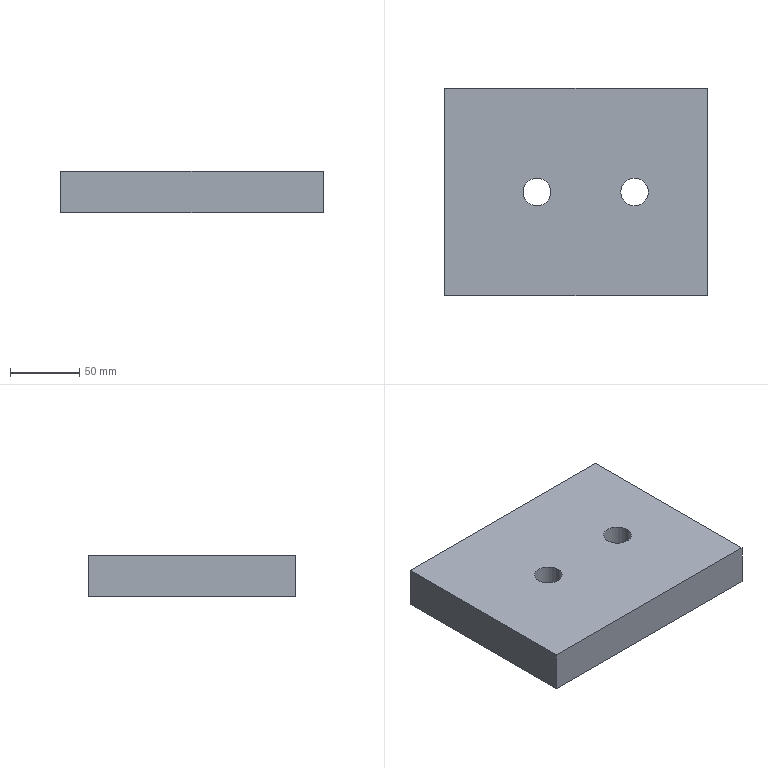Part | STEP file | 1 solid | 10 faces | box 190 x 150 x 30 mm | volume 836150 mm3 | plane 6 | cylinder 4 | commonest cylinder face diameters 20 x4
STEP:
#1=CARTESIAN_POINT('',(0.,0.,0.));
#2=DIRECTION('',(0.,0.,1.));
#3=DIRECTION('',(1.,0.,0.));
#4=AXIS2_PLACEMENT_3D('',#1,#2,#3);
#5=CARTESIAN_POINT('',(-38.283,0.,30.));
#6=VERTEX_POINT('',#5);
#7=CARTESIAN_POINT('',(-38.283,0.,0.));
#8=VERTEX_POINT('',#7);
#9=CARTESIAN_POINT('',(-38.283,0.,-49.));
#10=DIRECTION('',(0.,0.,-1.));
#11=VECTOR('',#10,1.);
#12=LINE('',#9,#11);
#13=CARTESIAN_POINT('',(-28.283,0.,-49.));
#14=DIRECTION('',(0.,0.,-1.));
#15=DIRECTION('',(-1.,0.,0.));
#16=AXIS2_PLACEMENT_3D('',#13,#14,#15);
#17=CYLINDRICAL_SURFACE('',#16,10.);
#18=CARTESIAN_POINT('',(6.283,0.));
#19=DIRECTION('',(0.,1.));
#20=VECTOR('',#19,1.);
#21=LINE('',#18,#20);
#22=(GEOMETRIC_REPRESENTATION_CONTEXT(2)PARAMETRIC_REPRESENTATION_CONTEXT()REPRESENTATION_CONTEXT('',''));
#23=DEFINITIONAL_REPRESENTATION('',(#21),#22);
#24=PCURVE('',#17,#23);
#25=CARTESIAN_POINT('',(-28.283,0.,-49.));
#26=DIRECTION('',(0.,0.,-1.));
#27=DIRECTION('',(-1.,0.,0.));
#28=AXIS2_PLACEMENT_3D('',#25,#26,#27);
#29=CYLINDRICAL_SURFACE('',#28,10.);
#30=CARTESIAN_POINT('',(0.,0.));
#31=DIRECTION('',(0.,1.));
#32=VECTOR('',#31,1.);
#33=LINE('',#30,#32);
#34=(GEOMETRIC_REPRESENTATION_CONTEXT(2)PARAMETRIC_REPRESENTATION_CONTEXT()REPRESENTATION_CONTEXT('',''));
#35=DEFINITIONAL_REPRESENTATION('',(#33),#34);
#36=PCURVE('',#29,#35);
#37=SURFACE_CURVE('',#12,(#24,#36),.PCURVE_S1.);
#38=EDGE_CURVE('',#6,#8,#37,.T.);
#39=ORIENTED_EDGE('',*,*,#38,.T.);
#40=CARTESIAN_POINT('',(-18.283,0.,0.));
#41=VERTEX_POINT('',#40);
#42=CARTESIAN_POINT('',(-28.283,0.,0.));
#43=DIRECTION('',(0.,0.,1.));
#44=DIRECTION('',(-1.,0.,0.));
#45=AXIS2_PLACEMENT_3D('',#42,#43,#44);
#46=CIRCLE('',#45,10.);
#47=CARTESIAN_POINT('',(6.283,-49.));
#48=DIRECTION('',(-1.,0.));
#49=VECTOR('',#48,1.);
#50=LINE('',#47,#49);
#51=(GEOMETRIC_REPRESENTATION_CONTEXT(2)PARAMETRIC_REPRESENTATION_CONTEXT()REPRESENTATION_CONTEXT('',''));
#52=DEFINITIONAL_REPRESENTATION('',(#50),#51);
#53=PCURVE('',#17,#52);
#54=CARTESIAN_POINT('',(0.,0.,0.));
#55=DIRECTION('',(0.,0.,1.));
#56=DIRECTION('',(1.,0.,0.));
#57=AXIS2_PLACEMENT_3D('',#54,#55,#56);
#58=PLANE('',#57);
#59=CARTESIAN_POINT('',(-28.283,0.));
#60=DIRECTION('',(-1.,0.));
#61=AXIS2_PLACEMENT_2D('',#59,#60);
#62=CIRCLE('',#61,10.);
#63=(GEOMETRIC_REPRESENTATION_CONTEXT(2)PARAMETRIC_REPRESENTATION_CONTEXT()REPRESENTATION_CONTEXT('',''));
#64=DEFINITIONAL_REPRESENTATION('',(#62),#63);
#65=PCURVE('',#58,#64);
#66=SURFACE_CURVE('',#46,(#53,#65),.PCURVE_S1.);
#67=EDGE_CURVE('',#8,#41,#66,.T.);
#68=ORIENTED_EDGE('',*,*,#67,.T.);
#69=CARTESIAN_POINT('',(-18.283,0.,30.));
#70=VERTEX_POINT('',#69);
#71=CARTESIAN_POINT('',(-18.283,0.,-49.));
#72=DIRECTION('',(0.,0.,-1.));
#73=VECTOR('',#72,1.);
#74=LINE('',#71,#73);
#75=CARTESIAN_POINT('',(3.142,0.));
#76=DIRECTION('',(0.,1.));
#77=VECTOR('',#76,1.);
#78=LINE('',#75,#77);
#79=(GEOMETRIC_REPRESENTATION_CONTEXT(2)PARAMETRIC_REPRESENTATION_CONTEXT()REPRESENTATION_CONTEXT('',''));
#80=DEFINITIONAL_REPRESENTATION('',(#78),#79);
#81=PCURVE('',#17,#80);
#82=CARTESIAN_POINT('',(3.142,0.));
#83=DIRECTION('',(0.,1.));
#84=VECTOR('',#83,1.);
#85=LINE('',#82,#84);
#86=(GEOMETRIC_REPRESENTATION_CONTEXT(2)PARAMETRIC_REPRESENTATION_CONTEXT()REPRESENTATION_CONTEXT('',''));
#87=DEFINITIONAL_REPRESENTATION('',(#85),#86);
#88=PCURVE('',#29,#87);
#89=SURFACE_CURVE('',#74,(#81,#88),.PCURVE_S1.);
#90=EDGE_CURVE('',#70,#41,#89,.T.);
#91=ORIENTED_EDGE('',*,*,#90,.F.);
#92=CARTESIAN_POINT('',(-28.283,0.,30.));
#93=DIRECTION('',(0.,0.,-1.));
#94=DIRECTION('',(-1.,0.,0.));
#95=AXIS2_PLACEMENT_3D('',#92,#93,#94);
#96=CIRCLE('',#95,10.);
#97=CARTESIAN_POINT('',(0.,-79.));
#98=DIRECTION('',(1.,0.));
#99=VECTOR('',#98,1.);
#100=LINE('',#97,#99);
#101=(GEOMETRIC_REPRESENTATION_CONTEXT(2)PARAMETRIC_REPRESENTATION_CONTEXT()REPRESENTATION_CONTEXT('',''));
#102=DEFINITIONAL_REPRESENTATION('',(#100),#101);
#103=PCURVE('',#17,#102);
#104=CARTESIAN_POINT('',(0.,0.,30.));
#105=DIRECTION('',(0.,0.,1.));
#106=DIRECTION('',(1.,0.,0.));
#107=AXIS2_PLACEMENT_3D('',#104,#105,#106);
#108=PLANE('',#107);
#109=CARTESIAN_POINT('',(-38.283,0.));
#110=CARTESIAN_POINT('',(-38.283,17.321));
#111=CARTESIAN_POINT('',(-23.283,8.66));
#112=CARTESIAN_POINT('',(-8.283,0.));
#113=CARTESIAN_POINT('',(-23.283,-8.66));
#114=CARTESIAN_POINT('',(-38.283,-17.321));
#115=CARTESIAN_POINT('',(-38.283,0.));
#116=(BOUNDED_CURVE()B_SPLINE_CURVE(2,(#109,#110,#111,#112,#113,#114,#115),.UNSPECIFIED.,.T.,.F.)B_SPLINE_CURVE_WITH_KNOTS((1,2,2,2,2,1),(-2.094,0.,2.094,4.189,6.283,8.378),.UNSPECIFIED.)CURVE()GEOMETRIC_REPRESENTATION_ITEM()RATIONAL_B_SPLINE_CURVE((1.,0.5,1.,0.5,1.,0.5,1.))REPRESENTATION_ITEM(''));
#117=(GEOMETRIC_REPRESENTATION_CONTEXT(2)PARAMETRIC_REPRESENTATION_CONTEXT()REPRESENTATION_CONTEXT('',''));
#118=DEFINITIONAL_REPRESENTATION('',(#116),#117);
#119=PCURVE('',#108,#118);
#120=SURFACE_CURVE('',#96,(#103,#119),.PCURVE_S1.);
#121=EDGE_CURVE('',#70,#6,#120,.T.);
#122=ORIENTED_EDGE('',*,*,#121,.T.);
#123=EDGE_LOOP('',(#39,#68,#91,#122));
#124=FACE_BOUND('',#123,.F.);
#125=ADVANCED_FACE('',(#124),#17,.F.);
#126=CARTESIAN_POINT('',(32.428,0.,30.));
#127=VERTEX_POINT('',#126);
#128=CARTESIAN_POINT('',(32.428,0.,0.));
#129=VERTEX_POINT('',#128);
#130=CARTESIAN_POINT('',(32.428,0.,-49.));
#131=DIRECTION('',(0.,0.,-1.));
#132=VECTOR('',#131,1.);
#133=LINE('',#130,#132);
#134=CARTESIAN_POINT('',(42.428,0.,-49.));
#135=DIRECTION('',(0.,0.,-1.));
#136=DIRECTION('',(-1.,0.,0.));
#137=AXIS2_PLACEMENT_3D('',#134,#135,#136);
#138=CYLINDRICAL_SURFACE('',#137,10.);
#139=CARTESIAN_POINT('',(6.283,0.));
#140=DIRECTION('',(0.,1.));
#141=VECTOR('',#140,1.);
#142=LINE('',#139,#141);
#143=(GEOMETRIC_REPRESENTATION_CONTEXT(2)PARAMETRIC_REPRESENTATION_CONTEXT()REPRESENTATION_CONTEXT('',''));
#144=DEFINITIONAL_REPRESENTATION('',(#142),#143);
#145=PCURVE('',#138,#144);
#146=CARTESIAN_POINT('',(42.428,0.,-49.));
#147=DIRECTION('',(0.,0.,-1.));
#148=DIRECTION('',(-1.,0.,0.));
#149=AXIS2_PLACEMENT_3D('',#146,#147,#148);
#150=CYLINDRICAL_SURFACE('',#149,10.);
#151=CARTESIAN_POINT('',(0.,0.));
#152=DIRECTION('',(0.,1.));
#153=VECTOR('',#152,1.);
#154=LINE('',#151,#153);
#155=(GEOMETRIC_REPRESENTATION_CONTEXT(2)PARAMETRIC_REPRESENTATION_CONTEXT()REPRESENTATION_CONTEXT('',''));
#156=DEFINITIONAL_REPRESENTATION('',(#154),#155);
#157=PCURVE('',#150,#156);
#158=SURFACE_CURVE('',#133,(#145,#157),.PCURVE_S1.);
#159=EDGE_CURVE('',#127,#129,#158,.T.);
#160=ORIENTED_EDGE('',*,*,#159,.T.);
#161=CARTESIAN_POINT('',(52.428,0.,0.));
#162=VERTEX_POINT('',#161);
#163=CARTESIAN_POINT('',(42.428,0.,0.));
#164=DIRECTION('',(0.,0.,1.));
#165=DIRECTION('',(-1.,0.,0.));
#166=AXIS2_PLACEMENT_3D('',#163,#164,#165);
#167=CIRCLE('',#166,10.);
#168=CARTESIAN_POINT('',(6.283,-49.));
#169=DIRECTION('',(-1.,0.));
#170=VECTOR('',#169,1.);
#171=LINE('',#168,#170);
#172=(GEOMETRIC_REPRESENTATION_CONTEXT(2)PARAMETRIC_REPRESENTATION_CONTEXT()REPRESENTATION_CONTEXT('',''));
#173=DEFINITIONAL_REPRESENTATION('',(#171),#172);
#174=PCURVE('',#138,#173);
#175=CARTESIAN_POINT('',(42.428,0.));
#176=DIRECTION('',(-1.,0.));
#177=AXIS2_PLACEMENT_2D('',#175,#176);
#178=CIRCLE('',#177,10.);
#179=(GEOMETRIC_REPRESENTATION_CONTEXT(2)PARAMETRIC_REPRESENTATION_CONTEXT()REPRESENTATION_CONTEXT('',''));
#180=DEFINITIONAL_REPRESENTATION('',(#178),#179);
#181=PCURVE('',#58,#180);
#182=SURFACE_CURVE('',#167,(#174,#181),.PCURVE_S1.);
#183=EDGE_CURVE('',#129,#162,#182,.T.);
#184=ORIENTED_EDGE('',*,*,#183,.T.);
#185=CARTESIAN_POINT('',(52.428,0.,30.));
#186=VERTEX_POINT('',#185);
#187=CARTESIAN_POINT('',(52.428,0.,-49.));
#188=DIRECTION('',(0.,0.,-1.));
#189=VECTOR('',#188,1.);
#190=LINE('',#187,#189);
#191=CARTESIAN_POINT('',(3.142,0.));
#192=DIRECTION('',(0.,1.));
#193=VECTOR('',#192,1.);
#194=LINE('',#191,#193);
#195=(GEOMETRIC_REPRESENTATION_CONTEXT(2)PARAMETRIC_REPRESENTATION_CONTEXT()REPRESENTATION_CONTEXT('',''));
#196=DEFINITIONAL_REPRESENTATION('',(#194),#195);
#197=PCURVE('',#138,#196);
#198=CARTESIAN_POINT('',(3.142,0.));
#199=DIRECTION('',(0.,1.));
#200=VECTOR('',#199,1.);
#201=LINE('',#198,#200);
#202=(GEOMETRIC_REPRESENTATION_CONTEXT(2)PARAMETRIC_REPRESENTATION_CONTEXT()REPRESENTATION_CONTEXT('',''));
#203=DEFINITIONAL_REPRESENTATION('',(#201),#202);
#204=PCURVE('',#150,#203);
#205=SURFACE_CURVE('',#190,(#197,#204),.PCURVE_S1.);
#206=EDGE_CURVE('',#186,#162,#205,.T.);
#207=ORIENTED_EDGE('',*,*,#206,.F.);
#208=CARTESIAN_POINT('',(42.428,0.,30.));
#209=DIRECTION('',(0.,0.,-1.));
#210=DIRECTION('',(-1.,0.,0.));
#211=AXIS2_PLACEMENT_3D('',#208,#209,#210);
#212=CIRCLE('',#211,10.);
#213=CARTESIAN_POINT('',(0.,-79.));
#214=DIRECTION('',(1.,0.));
#215=VECTOR('',#214,1.);
#216=LINE('',#213,#215);
#217=(GEOMETRIC_REPRESENTATION_CONTEXT(2)PARAMETRIC_REPRESENTATION_CONTEXT()REPRESENTATION_CONTEXT('',''));
#218=DEFINITIONAL_REPRESENTATION('',(#216),#217);
#219=PCURVE('',#138,#218);
#220=CARTESIAN_POINT('',(32.428,0.));
#221=CARTESIAN_POINT('',(32.428,17.321));
#222=CARTESIAN_POINT('',(47.428,8.66));
#223=CARTESIAN_POINT('',(62.428,0.));
#224=CARTESIAN_POINT('',(47.428,-8.66));
#225=CARTESIAN_POINT('',(32.428,-17.321));
#226=CARTESIAN_POINT('',(32.428,0.));
#227=(BOUNDED_CURVE()B_SPLINE_CURVE(2,(#220,#221,#222,#223,#224,#225,#226),.UNSPECIFIED.,.T.,.F.)B_SPLINE_CURVE_WITH_KNOTS((1,2,2,2,2,1),(-2.094,0.,2.094,4.189,6.283,8.378),.UNSPECIFIED.)CURVE()GEOMETRIC_REPRESENTATION_ITEM()RATIONAL_B_SPLINE_CURVE((1.,0.5,1.,0.5,1.,0.5,1.))REPRESENTATION_ITEM(''));
#228=(GEOMETRIC_REPRESENTATION_CONTEXT(2)PARAMETRIC_REPRESENTATION_CONTEXT()REPRESENTATION_CONTEXT('',''));
#229=DEFINITIONAL_REPRESENTATION('',(#227),#228);
#230=PCURVE('',#108,#229);
#231=SURFACE_CURVE('',#212,(#219,#230),.PCURVE_S1.);
#232=EDGE_CURVE('',#186,#127,#231,.T.);
#233=ORIENTED_EDGE('',*,*,#232,.T.);
#234=EDGE_LOOP('',(#160,#184,#207,#233));
#235=FACE_BOUND('',#234,.F.);
#236=ADVANCED_FACE('',(#235),#138,.F.);
#237=CARTESIAN_POINT('',(-28.283,0.,30.));
#238=DIRECTION('',(0.,0.,-1.));
#239=DIRECTION('',(-1.,0.,0.));
#240=AXIS2_PLACEMENT_3D('',#237,#238,#239);
#241=CIRCLE('',#240,10.);
#242=CARTESIAN_POINT('',(-38.283,0.));
#243=CARTESIAN_POINT('',(-38.283,17.321));
#244=CARTESIAN_POINT('',(-23.283,8.66));
#245=CARTESIAN_POINT('',(-8.283,0.));
#246=CARTESIAN_POINT('',(-23.283,-8.66));
#247=CARTESIAN_POINT('',(-38.283,-17.321));
#248=CARTESIAN_POINT('',(-38.283,0.));
#249=(BOUNDED_CURVE()B_SPLINE_CURVE(2,(#242,#243,#244,#245,#246,#247,#248),.UNSPECIFIED.,.T.,.F.)B_SPLINE_CURVE_WITH_KNOTS((1,2,2,2,2,1),(-2.094,0.,2.094,4.189,6.283,8.378),.UNSPECIFIED.)CURVE()GEOMETRIC_REPRESENTATION_ITEM()RATIONAL_B_SPLINE_CURVE((1.,0.5,1.,0.5,1.,0.5,1.))REPRESENTATION_ITEM(''));
#250=(GEOMETRIC_REPRESENTATION_CONTEXT(2)PARAMETRIC_REPRESENTATION_CONTEXT()REPRESENTATION_CONTEXT('',''));
#251=DEFINITIONAL_REPRESENTATION('',(#249),#250);
#252=PCURVE('',#108,#251);
#253=CARTESIAN_POINT('',(0.,-79.));
#254=DIRECTION('',(1.,0.));
#255=VECTOR('',#254,1.);
#256=LINE('',#253,#255);
#257=(GEOMETRIC_REPRESENTATION_CONTEXT(2)PARAMETRIC_REPRESENTATION_CONTEXT()REPRESENTATION_CONTEXT('',''));
#258=DEFINITIONAL_REPRESENTATION('',(#256),#257);
#259=PCURVE('',#29,#258);
#260=SURFACE_CURVE('',#241,(#252,#259),.PCURVE_S1.);
#261=EDGE_CURVE('',#6,#70,#260,.T.);
#262=ORIENTED_EDGE('',*,*,#261,.T.);
#263=ORIENTED_EDGE('',*,*,#121,.T.);
#264=EDGE_LOOP('',(#262,#263));
#265=FACE_BOUND('',#264,.T.);
#266=CARTESIAN_POINT('',(42.428,0.,30.));
#267=DIRECTION('',(0.,0.,-1.));
#268=DIRECTION('',(-1.,0.,0.));
#269=AXIS2_PLACEMENT_3D('',#266,#267,#268);
#270=CIRCLE('',#269,10.);
#271=CARTESIAN_POINT('',(32.428,0.));
#272=CARTESIAN_POINT('',(32.428,17.321));
#273=CARTESIAN_POINT('',(47.428,8.66));
#274=CARTESIAN_POINT('',(62.428,0.));
#275=CARTESIAN_POINT('',(47.428,-8.66));
#276=CARTESIAN_POINT('',(32.428,-17.321));
#277=CARTESIAN_POINT('',(32.428,0.));
#278=(BOUNDED_CURVE()B_SPLINE_CURVE(2,(#271,#272,#273,#274,#275,#276,#277),.UNSPECIFIED.,.T.,.F.)B_SPLINE_CURVE_WITH_KNOTS((1,2,2,2,2,1),(-2.094,0.,2.094,4.189,6.283,8.378),.UNSPECIFIED.)CURVE()GEOMETRIC_REPRESENTATION_ITEM()RATIONAL_B_SPLINE_CURVE((1.,0.5,1.,0.5,1.,0.5,1.))REPRESENTATION_ITEM(''));
#279=(GEOMETRIC_REPRESENTATION_CONTEXT(2)PARAMETRIC_REPRESENTATION_CONTEXT()REPRESENTATION_CONTEXT('',''));
#280=DEFINITIONAL_REPRESENTATION('',(#278),#279);
#281=PCURVE('',#108,#280);
#282=CARTESIAN_POINT('',(0.,-79.));
#283=DIRECTION('',(1.,0.));
#284=VECTOR('',#283,1.);
#285=LINE('',#282,#284);
#286=(GEOMETRIC_REPRESENTATION_CONTEXT(2)PARAMETRIC_REPRESENTATION_CONTEXT()REPRESENTATION_CONTEXT('',''));
#287=DEFINITIONAL_REPRESENTATION('',(#285),#286);
#288=PCURVE('',#150,#287);
#289=SURFACE_CURVE('',#270,(#281,#288),.PCURVE_S1.);
#290=EDGE_CURVE('',#127,#186,#289,.T.);
#291=ORIENTED_EDGE('',*,*,#290,.T.);
#292=ORIENTED_EDGE('',*,*,#232,.T.);
#293=EDGE_LOOP('',(#291,#292));
#294=FACE_BOUND('',#293,.T.);
#295=CARTESIAN_POINT('',(-95.,75.,30.));
#296=VERTEX_POINT('',#295);
#297=CARTESIAN_POINT('',(-95.,-75.,30.));
#298=VERTEX_POINT('',#297);
#299=CARTESIAN_POINT('',(-95.,0.,30.));
#300=DIRECTION('',(0.,-1.,0.));
#301=VECTOR('',#300,1.);
#302=LINE('',#299,#301);
#303=CARTESIAN_POINT('',(-95.,0.));
#304=DIRECTION('',(0.,-1.));
#305=VECTOR('',#304,1.);
#306=LINE('',#303,#305);
#307=(GEOMETRIC_REPRESENTATION_CONTEXT(2)PARAMETRIC_REPRESENTATION_CONTEXT()REPRESENTATION_CONTEXT('',''));
#308=DEFINITIONAL_REPRESENTATION('',(#306),#307);
#309=PCURVE('',#108,#308);
#310=CARTESIAN_POINT('',(-95.,75.,30.));
#311=DIRECTION('',(1.,0.,0.));
#312=DIRECTION('',(0.,1.,0.));
#313=AXIS2_PLACEMENT_3D('',#310,#311,#312);
#314=PLANE('',#313);
#315=CARTESIAN_POINT('',(-75.,0.));
#316=DIRECTION('',(-1.,0.));
#317=VECTOR('',#316,1.);
#318=LINE('',#315,#317);
#319=(GEOMETRIC_REPRESENTATION_CONTEXT(2)PARAMETRIC_REPRESENTATION_CONTEXT()REPRESENTATION_CONTEXT('',''));
#320=DEFINITIONAL_REPRESENTATION('',(#318),#319);
#321=PCURVE('',#314,#320);
#322=SURFACE_CURVE('',#302,(#309,#321),.PCURVE_S1.);
#323=EDGE_CURVE('',#296,#298,#322,.T.);
#324=ORIENTED_EDGE('',*,*,#323,.T.);
#325=CARTESIAN_POINT('',(95.,-75.,30.));
#326=VERTEX_POINT('',#325);
#327=CARTESIAN_POINT('',(0.,-75.,30.));
#328=DIRECTION('',(1.,0.,0.));
#329=VECTOR('',#328,1.);
#330=LINE('',#327,#329);
#331=CARTESIAN_POINT('',(0.,-75.));
#332=DIRECTION('',(1.,0.));
#333=VECTOR('',#332,1.);
#334=LINE('',#331,#333);
#335=(GEOMETRIC_REPRESENTATION_CONTEXT(2)PARAMETRIC_REPRESENTATION_CONTEXT()REPRESENTATION_CONTEXT('',''));
#336=DEFINITIONAL_REPRESENTATION('',(#334),#335);
#337=PCURVE('',#108,#336);
#338=CARTESIAN_POINT('',(-95.,-75.,30.));
#339=DIRECTION('',(0.,1.,0.));
#340=DIRECTION('',(0.,0.,1.));
#341=AXIS2_PLACEMENT_3D('',#338,#339,#340);
#342=PLANE('',#341);
#343=CARTESIAN_POINT('',(0.,95.));
#344=DIRECTION('',(0.,1.));
#345=VECTOR('',#344,1.);
#346=LINE('',#343,#345);
#347=(GEOMETRIC_REPRESENTATION_CONTEXT(2)PARAMETRIC_REPRESENTATION_CONTEXT()REPRESENTATION_CONTEXT('',''));
#348=DEFINITIONAL_REPRESENTATION('',(#346),#347);
#349=PCURVE('',#342,#348);
#350=SURFACE_CURVE('',#330,(#337,#349),.PCURVE_S1.);
#351=EDGE_CURVE('',#298,#326,#350,.T.);
#352=ORIENTED_EDGE('',*,*,#351,.T.);
#353=CARTESIAN_POINT('',(95.,75.,30.));
#354=VERTEX_POINT('',#353);
#355=CARTESIAN_POINT('',(95.,0.,30.));
#356=DIRECTION('',(0.,1.,0.));
#357=VECTOR('',#356,1.);
#358=LINE('',#355,#357);
#359=CARTESIAN_POINT('',(95.,0.));
#360=DIRECTION('',(0.,1.));
#361=VECTOR('',#360,1.);
#362=LINE('',#359,#361);
#363=(GEOMETRIC_REPRESENTATION_CONTEXT(2)PARAMETRIC_REPRESENTATION_CONTEXT()REPRESENTATION_CONTEXT('',''));
#364=DEFINITIONAL_REPRESENTATION('',(#362),#363);
#365=PCURVE('',#108,#364);
#366=CARTESIAN_POINT('',(95.,75.,30.));
#367=DIRECTION('',(-1.,0.,0.));
#368=DIRECTION('',(0.,0.,1.));
#369=AXIS2_PLACEMENT_3D('',#366,#367,#368);
#370=PLANE('',#369);
#371=CARTESIAN_POINT('',(0.,-75.));
#372=DIRECTION('',(0.,1.));
#373=VECTOR('',#372,1.);
#374=LINE('',#371,#373);
#375=(GEOMETRIC_REPRESENTATION_CONTEXT(2)PARAMETRIC_REPRESENTATION_CONTEXT()REPRESENTATION_CONTEXT('',''));
#376=DEFINITIONAL_REPRESENTATION('',(#374),#375);
#377=PCURVE('',#370,#376);
#378=SURFACE_CURVE('',#358,(#365,#377),.PCURVE_S1.);
#379=EDGE_CURVE('',#326,#354,#378,.T.);
#380=ORIENTED_EDGE('',*,*,#379,.T.);
#381=CARTESIAN_POINT('',(0.,75.,30.));
#382=DIRECTION('',(-1.,0.,0.));
#383=VECTOR('',#382,1.);
#384=LINE('',#381,#383);
#385=CARTESIAN_POINT('',(0.,75.));
#386=DIRECTION('',(-1.,0.));
#387=VECTOR('',#386,1.);
#388=LINE('',#385,#387);
#389=(GEOMETRIC_REPRESENTATION_CONTEXT(2)PARAMETRIC_REPRESENTATION_CONTEXT()REPRESENTATION_CONTEXT('',''));
#390=DEFINITIONAL_REPRESENTATION('',(#388),#389);
#391=PCURVE('',#108,#390);
#392=CARTESIAN_POINT('',(-95.,75.,30.));
#393=DIRECTION('',(0.,-1.,0.));
#394=DIRECTION('',(0.,0.,-1.));
#395=AXIS2_PLACEMENT_3D('',#392,#393,#394);
#396=PLANE('',#395);
#397=CARTESIAN_POINT('',(0.,95.));
#398=DIRECTION('',(0.,-1.));
#399=VECTOR('',#398,1.);
#400=LINE('',#397,#399);
#401=(GEOMETRIC_REPRESENTATION_CONTEXT(2)PARAMETRIC_REPRESENTATION_CONTEXT()REPRESENTATION_CONTEXT('',''));
#402=DEFINITIONAL_REPRESENTATION('',(#400),#401);
#403=PCURVE('',#396,#402);
#404=SURFACE_CURVE('',#384,(#391,#403),.PCURVE_S1.);
#405=EDGE_CURVE('',#354,#296,#404,.T.);
#406=ORIENTED_EDGE('',*,*,#405,.T.);
#407=EDGE_LOOP('',(#324,#352,#380,#406));
#408=FACE_BOUND('',#407,.T.);
#409=ADVANCED_FACE('',(#265,#294,#408),#108,.T.);
#410=CARTESIAN_POINT('',(-28.283,0.,0.));
#411=DIRECTION('',(0.,0.,1.));
#412=DIRECTION('',(-1.,0.,0.));
#413=AXIS2_PLACEMENT_3D('',#410,#411,#412);
#414=CIRCLE('',#413,10.);
#415=CARTESIAN_POINT('',(6.283,-49.));
#416=DIRECTION('',(-1.,0.));
#417=VECTOR('',#416,1.);
#418=LINE('',#415,#417);
#419=(GEOMETRIC_REPRESENTATION_CONTEXT(2)PARAMETRIC_REPRESENTATION_CONTEXT()REPRESENTATION_CONTEXT('',''));
#420=DEFINITIONAL_REPRESENTATION('',(#418),#419);
#421=PCURVE('',#29,#420);
#422=CARTESIAN_POINT('',(-28.283,0.));
#423=DIRECTION('',(-1.,0.));
#424=AXIS2_PLACEMENT_2D('',#422,#423);
#425=CIRCLE('',#424,10.);
#426=(GEOMETRIC_REPRESENTATION_CONTEXT(2)PARAMETRIC_REPRESENTATION_CONTEXT()REPRESENTATION_CONTEXT('',''));
#427=DEFINITIONAL_REPRESENTATION('',(#425),#426);
#428=PCURVE('',#58,#427);
#429=SURFACE_CURVE('',#414,(#421,#428),.PCURVE_S1.);
#430=EDGE_CURVE('',#41,#8,#429,.T.);
#431=ORIENTED_EDGE('',*,*,#430,.T.);
#432=ORIENTED_EDGE('',*,*,#38,.F.);
#433=ORIENTED_EDGE('',*,*,#261,.T.);
#434=ORIENTED_EDGE('',*,*,#90,.T.);
#435=EDGE_LOOP('',(#431,#432,#433,#434));
#436=FACE_BOUND('',#435,.F.);
#437=ADVANCED_FACE('',(#436),#29,.F.);
#438=CARTESIAN_POINT('',(42.428,0.,0.));
#439=DIRECTION('',(0.,0.,1.));
#440=DIRECTION('',(-1.,0.,0.));
#441=AXIS2_PLACEMENT_3D('',#438,#439,#440);
#442=CIRCLE('',#441,10.);
#443=CARTESIAN_POINT('',(6.283,-49.));
#444=DIRECTION('',(-1.,0.));
#445=VECTOR('',#444,1.);
#446=LINE('',#443,#445);
#447=(GEOMETRIC_REPRESENTATION_CONTEXT(2)PARAMETRIC_REPRESENTATION_CONTEXT()REPRESENTATION_CONTEXT('',''));
#448=DEFINITIONAL_REPRESENTATION('',(#446),#447);
#449=PCURVE('',#150,#448);
#450=CARTESIAN_POINT('',(42.428,0.));
#451=DIRECTION('',(-1.,0.));
#452=AXIS2_PLACEMENT_2D('',#450,#451);
#453=CIRCLE('',#452,10.);
#454=(GEOMETRIC_REPRESENTATION_CONTEXT(2)PARAMETRIC_REPRESENTATION_CONTEXT()REPRESENTATION_CONTEXT('',''));
#455=DEFINITIONAL_REPRESENTATION('',(#453),#454);
#456=PCURVE('',#58,#455);
#457=SURFACE_CURVE('',#442,(#449,#456),.PCURVE_S1.);
#458=EDGE_CURVE('',#162,#129,#457,.T.);
#459=ORIENTED_EDGE('',*,*,#458,.T.);
#460=ORIENTED_EDGE('',*,*,#159,.F.);
#461=ORIENTED_EDGE('',*,*,#290,.T.);
#462=ORIENTED_EDGE('',*,*,#206,.T.);
#463=EDGE_LOOP('',(#459,#460,#461,#462));
#464=FACE_BOUND('',#463,.F.);
#465=ADVANCED_FACE('',(#464),#150,.F.);
#466=CARTESIAN_POINT('',(95.,-75.,0.));
#467=VERTEX_POINT('',#466);
#468=CARTESIAN_POINT('',(95.,-75.,30.));
#469=DIRECTION('',(0.,0.,-1.));
#470=VECTOR('',#469,1.);
#471=LINE('',#468,#470);
#472=CARTESIAN_POINT('',(0.,190.));
#473=DIRECTION('',(-1.,0.));
#474=VECTOR('',#473,1.);
#475=LINE('',#472,#474);
#476=(GEOMETRIC_REPRESENTATION_CONTEXT(2)PARAMETRIC_REPRESENTATION_CONTEXT()REPRESENTATION_CONTEXT('',''));
#477=DEFINITIONAL_REPRESENTATION('',(#475),#476);
#478=PCURVE('',#342,#477);
#479=CARTESIAN_POINT('',(0.,-150.));
#480=DIRECTION('',(-1.,0.));
#481=VECTOR('',#480,1.);
#482=LINE('',#479,#481);
#483=(GEOMETRIC_REPRESENTATION_CONTEXT(2)PARAMETRIC_REPRESENTATION_CONTEXT()REPRESENTATION_CONTEXT('',''));
#484=DEFINITIONAL_REPRESENTATION('',(#482),#483);
#485=PCURVE('',#370,#484);
#486=SURFACE_CURVE('',#471,(#478,#485),.PCURVE_S1.);
#487=EDGE_CURVE('',#326,#467,#486,.T.);
#488=ORIENTED_EDGE('',*,*,#487,.F.);
#489=ORIENTED_EDGE('',*,*,#351,.F.);
#490=CARTESIAN_POINT('',(-95.,-75.,0.));
#491=VERTEX_POINT('',#490);
#492=CARTESIAN_POINT('',(-95.,-75.,30.));
#493=DIRECTION('',(0.,0.,1.));
#494=VECTOR('',#493,1.);
#495=LINE('',#492,#494);
#496=CARTESIAN_POINT('',(0.,0.));
#497=DIRECTION('',(1.,0.));
#498=VECTOR('',#497,1.);
#499=LINE('',#496,#498);
#500=(GEOMETRIC_REPRESENTATION_CONTEXT(2)PARAMETRIC_REPRESENTATION_CONTEXT()REPRESENTATION_CONTEXT('',''));
#501=DEFINITIONAL_REPRESENTATION('',(#499),#500);
#502=PCURVE('',#342,#501);
#503=CARTESIAN_POINT('',(-150.,0.));
#504=DIRECTION('',(0.,1.));
#505=VECTOR('',#504,1.);
#506=LINE('',#503,#505);
#507=(GEOMETRIC_REPRESENTATION_CONTEXT(2)PARAMETRIC_REPRESENTATION_CONTEXT()REPRESENTATION_CONTEXT('',''));
#508=DEFINITIONAL_REPRESENTATION('',(#506),#507);
#509=PCURVE('',#314,#508);
#510=SURFACE_CURVE('',#495,(#502,#509),.PCURVE_S1.);
#511=EDGE_CURVE('',#491,#298,#510,.T.);
#512=ORIENTED_EDGE('',*,*,#511,.F.);
#513=CARTESIAN_POINT('',(-95.,-75.,0.));
#514=DIRECTION('',(-1.,0.,0.));
#515=VECTOR('',#514,1.);
#516=LINE('',#513,#515);
#517=CARTESIAN_POINT('',(-30.,0.));
#518=DIRECTION('',(0.,-1.));
#519=VECTOR('',#518,1.);
#520=LINE('',#517,#519);
#521=(GEOMETRIC_REPRESENTATION_CONTEXT(2)PARAMETRIC_REPRESENTATION_CONTEXT()REPRESENTATION_CONTEXT('',''));
#522=DEFINITIONAL_REPRESENTATION('',(#520),#521);
#523=PCURVE('',#342,#522);
#524=CARTESIAN_POINT('',(-95.,-75.));
#525=DIRECTION('',(-1.,0.));
#526=VECTOR('',#525,1.);
#527=LINE('',#524,#526);
#528=(GEOMETRIC_REPRESENTATION_CONTEXT(2)PARAMETRIC_REPRESENTATION_CONTEXT()REPRESENTATION_CONTEXT('',''));
#529=DEFINITIONAL_REPRESENTATION('',(#527),#528);
#530=PCURVE('',#58,#529);
#531=SURFACE_CURVE('',#516,(#523,#530),.PCURVE_S1.);
#532=EDGE_CURVE('',#467,#491,#531,.T.);
#533=ORIENTED_EDGE('',*,*,#532,.F.);
#534=EDGE_LOOP('',(#488,#489,#512,#533));
#535=FACE_BOUND('',#534,.T.);
#536=ADVANCED_FACE('',(#535),#342,.F.);
#537=ORIENTED_EDGE('',*,*,#511,.T.);
#538=ORIENTED_EDGE('',*,*,#323,.F.);
#539=CARTESIAN_POINT('',(-95.,75.,0.));
#540=VERTEX_POINT('',#539);
#541=CARTESIAN_POINT('',(-95.,75.,30.));
#542=DIRECTION('',(0.,0.,1.));
#543=VECTOR('',#542,1.);
#544=LINE('',#541,#543);
#545=CARTESIAN_POINT('',(0.,0.));
#546=DIRECTION('',(0.,1.));
#547=VECTOR('',#546,1.);
#548=LINE('',#545,#547);
#549=(GEOMETRIC_REPRESENTATION_CONTEXT(2)PARAMETRIC_REPRESENTATION_CONTEXT()REPRESENTATION_CONTEXT('',''));
#550=DEFINITIONAL_REPRESENTATION('',(#548),#549);
#551=PCURVE('',#314,#550);
#552=CARTESIAN_POINT('',(0.,0.));
#553=DIRECTION('',(-1.,0.));
#554=VECTOR('',#553,1.);
#555=LINE('',#552,#554);
#556=(GEOMETRIC_REPRESENTATION_CONTEXT(2)PARAMETRIC_REPRESENTATION_CONTEXT()REPRESENTATION_CONTEXT('',''));
#557=DEFINITIONAL_REPRESENTATION('',(#555),#556);
#558=PCURVE('',#396,#557);
#559=SURFACE_CURVE('',#544,(#551,#558),.PCURVE_S1.);
#560=EDGE_CURVE('',#540,#296,#559,.T.);
#561=ORIENTED_EDGE('',*,*,#560,.F.);
#562=CARTESIAN_POINT('',(-95.,75.,0.));
#563=DIRECTION('',(0.,1.,0.));
#564=VECTOR('',#563,1.);
#565=LINE('',#562,#564);
#566=CARTESIAN_POINT('',(0.,-30.));
#567=DIRECTION('',(1.,0.));
#568=VECTOR('',#567,1.);
#569=LINE('',#566,#568);
#570=(GEOMETRIC_REPRESENTATION_CONTEXT(2)PARAMETRIC_REPRESENTATION_CONTEXT()REPRESENTATION_CONTEXT('',''));
#571=DEFINITIONAL_REPRESENTATION('',(#569),#570);
#572=PCURVE('',#314,#571);
#573=CARTESIAN_POINT('',(-95.,75.));
#574=DIRECTION('',(0.,1.));
#575=VECTOR('',#574,1.);
#576=LINE('',#573,#575);
#577=(GEOMETRIC_REPRESENTATION_CONTEXT(2)PARAMETRIC_REPRESENTATION_CONTEXT()REPRESENTATION_CONTEXT('',''));
#578=DEFINITIONAL_REPRESENTATION('',(#576),#577);
#579=PCURVE('',#58,#578);
#580=SURFACE_CURVE('',#565,(#572,#579),.PCURVE_S1.);
#581=EDGE_CURVE('',#491,#540,#580,.T.);
#582=ORIENTED_EDGE('',*,*,#581,.F.);
#583=EDGE_LOOP('',(#537,#538,#561,#582));
#584=FACE_BOUND('',#583,.T.);
#585=ADVANCED_FACE('',(#584),#314,.F.);
#586=ORIENTED_EDGE('',*,*,#560,.T.);
#587=ORIENTED_EDGE('',*,*,#405,.F.);
#588=CARTESIAN_POINT('',(95.,75.,0.));
#589=VERTEX_POINT('',#588);
#590=CARTESIAN_POINT('',(95.,75.,30.));
#591=DIRECTION('',(0.,0.,1.));
#592=VECTOR('',#591,1.);
#593=LINE('',#590,#592);
#594=CARTESIAN_POINT('',(0.,190.));
#595=DIRECTION('',(-1.,0.));
#596=VECTOR('',#595,1.);
#597=LINE('',#594,#596);
#598=(GEOMETRIC_REPRESENTATION_CONTEXT(2)PARAMETRIC_REPRESENTATION_CONTEXT()REPRESENTATION_CONTEXT('',''));
#599=DEFINITIONAL_REPRESENTATION('',(#597),#598);
#600=PCURVE('',#396,#599);
#601=CARTESIAN_POINT('',(0.,0.));
#602=DIRECTION('',(1.,0.));
#603=VECTOR('',#602,1.);
#604=LINE('',#601,#603);
#605=(GEOMETRIC_REPRESENTATION_CONTEXT(2)PARAMETRIC_REPRESENTATION_CONTEXT()REPRESENTATION_CONTEXT('',''));
#606=DEFINITIONAL_REPRESENTATION('',(#604),#605);
#607=PCURVE('',#370,#606);
#608=SURFACE_CURVE('',#593,(#600,#607),.PCURVE_S1.);
#609=EDGE_CURVE('',#589,#354,#608,.T.);
#610=ORIENTED_EDGE('',*,*,#609,.F.);
#611=CARTESIAN_POINT('',(-95.,75.,0.));
#612=DIRECTION('',(1.,0.,0.));
#613=VECTOR('',#612,1.);
#614=LINE('',#611,#613);
#615=CARTESIAN_POINT('',(30.,0.));
#616=DIRECTION('',(0.,1.));
#617=VECTOR('',#616,1.);
#618=LINE('',#615,#617);
#619=(GEOMETRIC_REPRESENTATION_CONTEXT(2)PARAMETRIC_REPRESENTATION_CONTEXT()REPRESENTATION_CONTEXT('',''));
#620=DEFINITIONAL_REPRESENTATION('',(#618),#619);
#621=PCURVE('',#396,#620);
#622=CARTESIAN_POINT('',(-95.,75.));
#623=DIRECTION('',(1.,0.));
#624=VECTOR('',#623,1.);
#625=LINE('',#622,#624);
#626=(GEOMETRIC_REPRESENTATION_CONTEXT(2)PARAMETRIC_REPRESENTATION_CONTEXT()REPRESENTATION_CONTEXT('',''));
#627=DEFINITIONAL_REPRESENTATION('',(#625),#626);
#628=PCURVE('',#58,#627);
#629=SURFACE_CURVE('',#614,(#621,#628),.PCURVE_S1.);
#630=EDGE_CURVE('',#540,#589,#629,.T.);
#631=ORIENTED_EDGE('',*,*,#630,.F.);
#632=EDGE_LOOP('',(#586,#587,#610,#631));
#633=FACE_BOUND('',#632,.T.);
#634=ADVANCED_FACE('',(#633),#396,.F.);
#635=ORIENTED_EDGE('',*,*,#609,.T.);
#636=ORIENTED_EDGE('',*,*,#379,.F.);
#637=ORIENTED_EDGE('',*,*,#487,.T.);
#638=CARTESIAN_POINT('',(95.,75.,0.));
#639=DIRECTION('',(0.,-1.,0.));
#640=VECTOR('',#639,1.);
#641=LINE('',#638,#640);
#642=CARTESIAN_POINT('',(-30.,0.));
#643=DIRECTION('',(0.,-1.));
#644=VECTOR('',#643,1.);
#645=LINE('',#642,#644);
#646=(GEOMETRIC_REPRESENTATION_CONTEXT(2)PARAMETRIC_REPRESENTATION_CONTEXT()REPRESENTATION_CONTEXT('',''));
#647=DEFINITIONAL_REPRESENTATION('',(#645),#646);
#648=PCURVE('',#370,#647);
#649=CARTESIAN_POINT('',(95.,75.));
#650=DIRECTION('',(0.,-1.));
#651=VECTOR('',#650,1.);
#652=LINE('',#649,#651);
#653=(GEOMETRIC_REPRESENTATION_CONTEXT(2)PARAMETRIC_REPRESENTATION_CONTEXT()REPRESENTATION_CONTEXT('',''));
#654=DEFINITIONAL_REPRESENTATION('',(#652),#653);
#655=PCURVE('',#58,#654);
#656=SURFACE_CURVE('',#641,(#648,#655),.PCURVE_S1.);
#657=EDGE_CURVE('',#589,#467,#656,.T.);
#658=ORIENTED_EDGE('',*,*,#657,.F.);
#659=EDGE_LOOP('',(#635,#636,#637,#658));
#660=FACE_BOUND('',#659,.T.);
#661=ADVANCED_FACE('',(#660),#370,.F.);
#662=ORIENTED_EDGE('',*,*,#67,.T.);
#663=ORIENTED_EDGE('',*,*,#430,.T.);
#664=EDGE_LOOP('',(#662,#663));
#665=FACE_BOUND('',#664,.T.);
#666=ORIENTED_EDGE('',*,*,#183,.T.);
#667=ORIENTED_EDGE('',*,*,#458,.T.);
#668=EDGE_LOOP('',(#666,#667));
#669=FACE_BOUND('',#668,.T.);
#670=ORIENTED_EDGE('',*,*,#532,.T.);
#671=ORIENTED_EDGE('',*,*,#581,.T.);
#672=ORIENTED_EDGE('',*,*,#630,.T.);
#673=ORIENTED_EDGE('',*,*,#657,.T.);
#674=EDGE_LOOP('',(#670,#671,#672,#673));
#675=FACE_BOUND('',#674,.T.);
#676=ADVANCED_FACE('',(#665,#669,#675),#58,.F.);
#677=CLOSED_SHELL('',(#125,#236,#409,#437,#465,#536,#585,#634,#661,#676));
#678=MANIFOLD_SOLID_BREP('',#677);
#679=(LENGTH_UNIT()NAMED_UNIT(*)SI_UNIT(.MILLI.,.METRE.));
#680=UNCERTAINTY_MEASURE_WITH_UNIT(LENGTH_MEASURE(0.0000001),#679,'','');
#681=(NAMED_UNIT(*)PLANE_ANGLE_UNIT()SI_UNIT($,.RADIAN.));
#682=(NAMED_UNIT(*)SI_UNIT($,.STERADIAN.)SOLID_ANGLE_UNIT());
#683=(GEOMETRIC_REPRESENTATION_CONTEXT(3)GLOBAL_UNCERTAINTY_ASSIGNED_CONTEXT((#680))GLOBAL_UNIT_ASSIGNED_CONTEXT((#679,#681,#682))REPRESENTATION_CONTEXT('',''));
#684=ADVANCED_BREP_SHAPE_REPRESENTATION('',(#4,#678),#683);